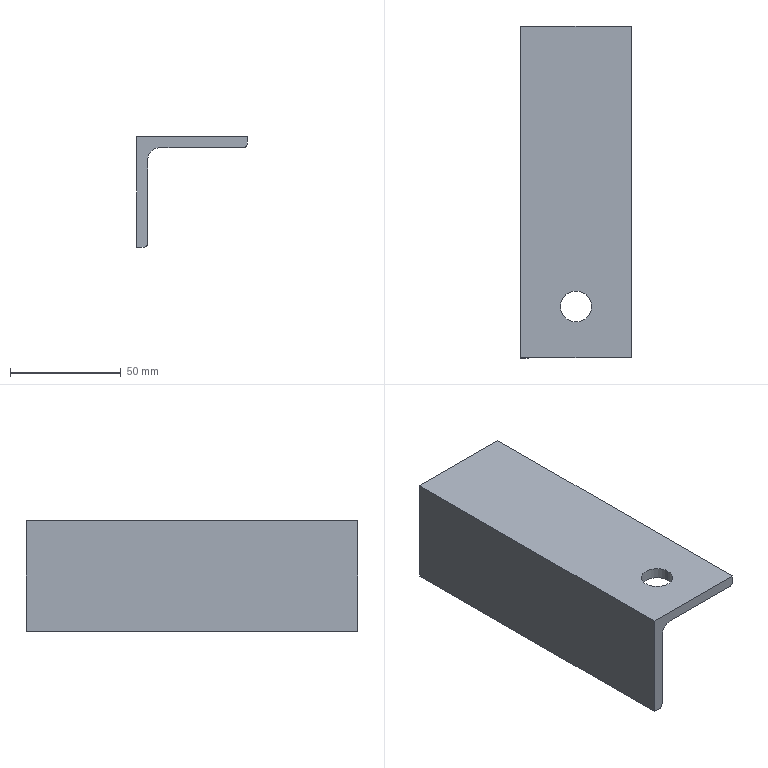Part | SolidWorks | features BaseBody 1 | 1 solid | 13 faces | box 50 x 150 x 50 mm | volume 71275 mm3 | plane 8 | cylinder 5 | commonest cylinder face diameters 3.333 x2 14 x2 11 x1
STEP:
#1=CARTESIAN_POINT('',(32.,-126.8,-5.));
#2=VERTEX_POINT('',#1);
#3=CARTESIAN_POINT('',(18.,-126.8,-5.));
#4=VERTEX_POINT('',#3);
#5=CARTESIAN_POINT('',(25.,-126.8,-5.));
#6=DIRECTION('',(0.,0.,-1.));
#7=DIRECTION('',(1.,0.,0.));
#8=AXIS2_PLACEMENT_3D('',#5,#6,#7);
#9=CIRCLE('',#8,7.);
#10=EDGE_CURVE('',#2,#4,#9,.T.);
#11=ORIENTED_EDGE('',*,*,#10,.T.);
#12=CARTESIAN_POINT('',(18.,-126.8,0.));
#13=VERTEX_POINT('',#12);
#14=CARTESIAN_POINT('',(18.,-126.8,-10.));
#15=DIRECTION('',(0.,0.,1.));
#16=VECTOR('',#15,1000.);
#17=LINE('',#14,#16);
#18=EDGE_CURVE('',#4,#13,#17,.T.);
#19=ORIENTED_EDGE('',*,*,#18,.T.);
#20=CARTESIAN_POINT('',(32.,-126.8,0.));
#21=VERTEX_POINT('',#20);
#22=CARTESIAN_POINT('',(25.,-126.8,0.));
#23=DIRECTION('',(0.,0.,1.));
#24=DIRECTION('',(1.,0.,0.));
#25=AXIS2_PLACEMENT_3D('',#22,#23,#24);
#26=CIRCLE('',#25,7.);
#27=EDGE_CURVE('',#13,#21,#26,.T.);
#28=ORIENTED_EDGE('',*,*,#27,.T.);
#29=CARTESIAN_POINT('',(32.,-126.8,-10.));
#30=DIRECTION('',(0.,0.,1.));
#31=VECTOR('',#30,1000.);
#32=LINE('',#29,#31);
#33=EDGE_CURVE('',#2,#21,#32,.T.);
#34=ORIENTED_EDGE('',*,*,#33,.F.);
#35=EDGE_LOOP('',(#11,#19,#28,#34));
#36=FACE_OUTER_BOUND('',#35,.T.);
#37=CARTESIAN_POINT('',(25.,-126.8,-10.));
#38=DIRECTION('',(0.,0.,1.));
#39=DIRECTION('',(1.,0.,0.));
#40=AXIS2_PLACEMENT_3D('',#37,#38,#39);
#41=CYLINDRICAL_SURFACE('',#40,7.);
#42=ADVANCED_FACE('',(#36),#41,.F.);
#43=CARTESIAN_POINT('',(0.,-150.,-50.));
#44=VERTEX_POINT('',#43);
#45=CARTESIAN_POINT('',(0.,0.,-50.));
#46=VERTEX_POINT('',#45);
#47=CARTESIAN_POINT('',(0.,-150.,-50.));
#48=DIRECTION('',(0.,1.,0.));
#49=VECTOR('',#48,1000.);
#50=LINE('',#47,#49);
#51=EDGE_CURVE('',#44,#46,#50,.T.);
#52=ORIENTED_EDGE('',*,*,#51,.F.);
#53=CARTESIAN_POINT('',(0.,-150.,0.));
#54=VERTEX_POINT('',#53);
#55=CARTESIAN_POINT('',(0.,-150.,0.));
#56=DIRECTION('',(0.,0.,-1.));
#57=VECTOR('',#56,1000.);
#58=LINE('',#55,#57);
#59=EDGE_CURVE('',#54,#44,#58,.T.);
#60=ORIENTED_EDGE('',*,*,#59,.F.);
#61=CARTESIAN_POINT('',(0.,0.,0.));
#62=VERTEX_POINT('',#61);
#63=CARTESIAN_POINT('',(0.,-150.,0.));
#64=DIRECTION('',(0.,-1.,0.));
#65=VECTOR('',#64,1000.);
#66=LINE('',#63,#65);
#67=EDGE_CURVE('',#62,#54,#66,.T.);
#68=ORIENTED_EDGE('',*,*,#67,.F.);
#69=CARTESIAN_POINT('',(0.,0.,0.));
#70=DIRECTION('',(0.,0.,1.));
#71=VECTOR('',#70,1000.);
#72=LINE('',#69,#71);
#73=EDGE_CURVE('',#46,#62,#72,.T.);
#74=ORIENTED_EDGE('',*,*,#73,.F.);
#75=EDGE_LOOP('',(#52,#60,#68,#74));
#76=FACE_OUTER_BOUND('',#75,.T.);
#77=CARTESIAN_POINT('',(0.,-150.,0.));
#78=DIRECTION('',(1.,0.,0.));
#79=DIRECTION('',(0.,1.,0.));
#80=AXIS2_PLACEMENT_3D('',#77,#78,#79);
#81=PLANE('',#80);
#82=ADVANCED_FACE('',(#76),#81,.F.);
#83=ORIENTED_EDGE('',*,*,#73,.T.);
#84=CARTESIAN_POINT('',(50.,0.,0.));
#85=VERTEX_POINT('',#84);
#86=CARTESIAN_POINT('',(48.333,0.,0.));
#87=DIRECTION('',(1.,0.,0.));
#88=VECTOR('',#87,1000.);
#89=LINE('',#86,#88);
#90=EDGE_CURVE('',#62,#85,#89,.T.);
#91=ORIENTED_EDGE('',*,*,#90,.T.);
#92=CARTESIAN_POINT('',(50.,0.,-3.333));
#93=VERTEX_POINT('',#92);
#94=CARTESIAN_POINT('',(50.,0.,-3.333));
#95=DIRECTION('',(0.,0.,-1.));
#96=VECTOR('',#95,1000.);
#97=LINE('',#94,#96);
#98=EDGE_CURVE('',#85,#93,#97,.T.);
#99=ORIENTED_EDGE('',*,*,#98,.T.);
#100=CARTESIAN_POINT('',(48.333,0.,-5.));
#101=VERTEX_POINT('',#100);
#102=CARTESIAN_POINT('',(48.333,0.,-3.333));
#103=DIRECTION('',(0.,1.,0.));
#104=DIRECTION('',(-1.,0.,0.));
#105=AXIS2_PLACEMENT_3D('',#102,#103,#104);
#106=CIRCLE('',#105,1.667);
#107=EDGE_CURVE('',#93,#101,#106,.T.);
#108=ORIENTED_EDGE('',*,*,#107,.T.);
#109=CARTESIAN_POINT('',(10.5,0.,-5.));
#110=VERTEX_POINT('',#109);
#111=CARTESIAN_POINT('',(48.333,0.,-5.));
#112=DIRECTION('',(-1.,0.,0.));
#113=VECTOR('',#112,1000.);
#114=LINE('',#111,#113);
#115=EDGE_CURVE('',#101,#110,#114,.T.);
#116=ORIENTED_EDGE('',*,*,#115,.T.);
#117=CARTESIAN_POINT('',(5.,0.,-10.5));
#118=VERTEX_POINT('',#117);
#119=CARTESIAN_POINT('',(10.5,0.,-10.5));
#120=DIRECTION('',(0.,-1.,0.));
#121=DIRECTION('',(-1.,0.,0.));
#122=AXIS2_PLACEMENT_3D('',#119,#120,#121);
#123=CIRCLE('',#122,5.5);
#124=EDGE_CURVE('',#110,#118,#123,.T.);
#125=ORIENTED_EDGE('',*,*,#124,.T.);
#126=CARTESIAN_POINT('',(5.,0.,-48.333));
#127=VERTEX_POINT('',#126);
#128=CARTESIAN_POINT('',(5.,0.,-3.333));
#129=DIRECTION('',(0.,0.,-1.));
#130=VECTOR('',#129,1000.);
#131=LINE('',#128,#130);
#132=EDGE_CURVE('',#118,#127,#131,.T.);
#133=ORIENTED_EDGE('',*,*,#132,.T.);
#134=CARTESIAN_POINT('',(3.333,0.,-50.));
#135=VERTEX_POINT('',#134);
#136=CARTESIAN_POINT('',(3.333,0.,-48.333));
#137=DIRECTION('',(0.,1.,0.));
#138=DIRECTION('',(-1.,0.,0.));
#139=AXIS2_PLACEMENT_3D('',#136,#137,#138);
#140=CIRCLE('',#139,1.667);
#141=EDGE_CURVE('',#127,#135,#140,.T.);
#142=ORIENTED_EDGE('',*,*,#141,.T.);
#143=CARTESIAN_POINT('',(48.333,0.,-50.));
#144=DIRECTION('',(-1.,0.,0.));
#145=VECTOR('',#144,1000.);
#146=LINE('',#143,#145);
#147=EDGE_CURVE('',#135,#46,#146,.T.);
#148=ORIENTED_EDGE('',*,*,#147,.T.);
#149=EDGE_LOOP('',(#83,#91,#99,#108,#116,#125,#133,#142,#148));
#150=FACE_OUTER_BOUND('',#149,.T.);
#151=CARTESIAN_POINT('',(48.333,0.,-3.333));
#152=DIRECTION('',(0.,1.,0.));
#153=DIRECTION('',(-1.,0.,0.));
#154=AXIS2_PLACEMENT_3D('',#151,#152,#153);
#155=PLANE('',#154);
#156=ADVANCED_FACE('',(#150),#155,.T.);
#157=CARTESIAN_POINT('',(3.333,-150.,-50.));
#158=VERTEX_POINT('',#157);
#159=CARTESIAN_POINT('',(3.333,-150.,-50.));
#160=DIRECTION('',(0.,1.,0.));
#161=VECTOR('',#160,1000.);
#162=LINE('',#159,#161);
#163=EDGE_CURVE('',#158,#135,#162,.T.);
#164=ORIENTED_EDGE('',*,*,#163,.F.);
#165=CARTESIAN_POINT('',(0.,-150.,-50.));
#166=DIRECTION('',(1.,0.,0.));
#167=VECTOR('',#166,1000.);
#168=LINE('',#165,#167);
#169=EDGE_CURVE('',#44,#158,#168,.T.);
#170=ORIENTED_EDGE('',*,*,#169,.F.);
#171=ORIENTED_EDGE('',*,*,#51,.T.);
#172=ORIENTED_EDGE('',*,*,#147,.F.);
#173=EDGE_LOOP('',(#164,#170,#171,#172));
#174=FACE_OUTER_BOUND('',#173,.T.);
#175=CARTESIAN_POINT('',(0.,-150.,-50.));
#176=DIRECTION('',(0.,0.,1.));
#177=DIRECTION('',(1.,0.,0.));
#178=AXIS2_PLACEMENT_3D('',#175,#176,#177);
#179=PLANE('',#178);
#180=ADVANCED_FACE('',(#174),#179,.F.);
#181=CARTESIAN_POINT('',(50.,-150.,0.));
#182=VERTEX_POINT('',#181);
#183=CARTESIAN_POINT('',(48.333,-150.,0.));
#184=DIRECTION('',(1.,0.,0.));
#185=VECTOR('',#184,1000.);
#186=LINE('',#183,#185);
#187=EDGE_CURVE('',#54,#182,#186,.T.);
#188=ORIENTED_EDGE('',*,*,#187,.F.);
#189=ORIENTED_EDGE('',*,*,#59,.T.);
#190=ORIENTED_EDGE('',*,*,#169,.T.);
#191=CARTESIAN_POINT('',(5.,-150.,-48.333));
#192=VERTEX_POINT('',#191);
#193=CARTESIAN_POINT('',(3.333,-150.,-48.333));
#194=DIRECTION('',(0.,1.,0.));
#195=DIRECTION('',(-1.,0.,0.));
#196=AXIS2_PLACEMENT_3D('',#193,#194,#195);
#197=CIRCLE('',#196,1.667);
#198=EDGE_CURVE('',#192,#158,#197,.T.);
#199=ORIENTED_EDGE('',*,*,#198,.F.);
#200=CARTESIAN_POINT('',(5.,-150.,-10.5));
#201=VERTEX_POINT('',#200);
#202=CARTESIAN_POINT('',(5.,-150.,-3.333));
#203=DIRECTION('',(0.,0.,-1.));
#204=VECTOR('',#203,1000.);
#205=LINE('',#202,#204);
#206=EDGE_CURVE('',#201,#192,#205,.T.);
#207=ORIENTED_EDGE('',*,*,#206,.F.);
#208=CARTESIAN_POINT('',(10.5,-150.,-5.));
#209=VERTEX_POINT('',#208);
#210=CARTESIAN_POINT('',(10.5,-150.,-10.5));
#211=DIRECTION('',(0.,-1.,0.));
#212=DIRECTION('',(-1.,0.,0.));
#213=AXIS2_PLACEMENT_3D('',#210,#211,#212);
#214=CIRCLE('',#213,5.5);
#215=EDGE_CURVE('',#209,#201,#214,.T.);
#216=ORIENTED_EDGE('',*,*,#215,.F.);
#217=CARTESIAN_POINT('',(48.333,-150.,-5.));
#218=VERTEX_POINT('',#217);
#219=CARTESIAN_POINT('',(48.333,-150.,-5.));
#220=DIRECTION('',(-1.,0.,0.));
#221=VECTOR('',#220,1000.);
#222=LINE('',#219,#221);
#223=EDGE_CURVE('',#218,#209,#222,.T.);
#224=ORIENTED_EDGE('',*,*,#223,.F.);
#225=CARTESIAN_POINT('',(50.,-150.,-3.333));
#226=VERTEX_POINT('',#225);
#227=CARTESIAN_POINT('',(48.333,-150.,-3.333));
#228=DIRECTION('',(0.,1.,0.));
#229=DIRECTION('',(-1.,0.,0.));
#230=AXIS2_PLACEMENT_3D('',#227,#228,#229);
#231=CIRCLE('',#230,1.667);
#232=EDGE_CURVE('',#226,#218,#231,.T.);
#233=ORIENTED_EDGE('',*,*,#232,.F.);
#234=CARTESIAN_POINT('',(50.,-150.,-3.333));
#235=DIRECTION('',(0.,0.,-1.));
#236=VECTOR('',#235,1000.);
#237=LINE('',#234,#236);
#238=EDGE_CURVE('',#182,#226,#237,.T.);
#239=ORIENTED_EDGE('',*,*,#238,.F.);
#240=EDGE_LOOP('',(#188,#189,#190,#199,#207,#216,#224,#233,#239));
#241=FACE_OUTER_BOUND('',#240,.T.);
#242=CARTESIAN_POINT('',(48.333,-150.,-3.333));
#243=DIRECTION('',(0.,1.,0.));
#244=DIRECTION('',(-1.,0.,0.));
#245=AXIS2_PLACEMENT_3D('',#242,#243,#244);
#246=PLANE('',#245);
#247=ADVANCED_FACE('',(#241),#246,.F.);
#248=ORIENTED_EDGE('',*,*,#67,.T.);
#249=ORIENTED_EDGE('',*,*,#187,.T.);
#250=CARTESIAN_POINT('',(50.,-150.,0.));
#251=DIRECTION('',(0.,-1.,0.));
#252=VECTOR('',#251,1000.);
#253=LINE('',#250,#252);
#254=EDGE_CURVE('',#85,#182,#253,.T.);
#255=ORIENTED_EDGE('',*,*,#254,.F.);
#256=ORIENTED_EDGE('',*,*,#90,.F.);
#257=EDGE_LOOP('',(#248,#249,#255,#256));
#258=FACE_OUTER_BOUND('',#257,.T.);
#259=CARTESIAN_POINT('',(25.,-126.8,0.));
#260=DIRECTION('',(0.,0.,1.));
#261=DIRECTION('',(1.,0.,0.));
#262=AXIS2_PLACEMENT_3D('',#259,#260,#261);
#263=CIRCLE('',#262,7.);
#264=EDGE_CURVE('',#21,#13,#263,.T.);
#265=ORIENTED_EDGE('',*,*,#264,.F.);
#266=ORIENTED_EDGE('',*,*,#27,.F.);
#267=EDGE_LOOP('',(#265,#266));
#268=FACE_BOUND('',#267,.T.);
#269=CARTESIAN_POINT('',(50.,-150.,0.));
#270=DIRECTION('',(0.,0.,-1.));
#271=DIRECTION('',(-1.,0.,0.));
#272=AXIS2_PLACEMENT_3D('',#269,#270,#271);
#273=PLANE('',#272);
#274=ADVANCED_FACE('',(#258,#268),#273,.F.);
#275=ORIENTED_EDGE('',*,*,#198,.T.);
#276=ORIENTED_EDGE('',*,*,#163,.T.);
#277=ORIENTED_EDGE('',*,*,#141,.F.);
#278=CARTESIAN_POINT('',(5.,-150.,-48.333));
#279=DIRECTION('',(0.,-1.,0.));
#280=VECTOR('',#279,1000.);
#281=LINE('',#278,#280);
#282=EDGE_CURVE('',#127,#192,#281,.T.);
#283=ORIENTED_EDGE('',*,*,#282,.T.);
#284=EDGE_LOOP('',(#275,#276,#277,#283));
#285=FACE_OUTER_BOUND('',#284,.T.);
#286=CARTESIAN_POINT('',(3.333,-150.,-48.333));
#287=DIRECTION('',(0.,1.,0.));
#288=DIRECTION('',(-1.,0.,0.));
#289=AXIS2_PLACEMENT_3D('',#286,#287,#288);
#290=CYLINDRICAL_SURFACE('',#289,1.667);
#291=ADVANCED_FACE('',(#285),#290,.T.);
#292=CARTESIAN_POINT('',(5.,-150.,-10.5));
#293=DIRECTION('',(0.,1.,0.));
#294=VECTOR('',#293,1000.);
#295=LINE('',#292,#294);
#296=EDGE_CURVE('',#201,#118,#295,.T.);
#297=ORIENTED_EDGE('',*,*,#296,.F.);
#298=ORIENTED_EDGE('',*,*,#206,.T.);
#299=ORIENTED_EDGE('',*,*,#282,.F.);
#300=ORIENTED_EDGE('',*,*,#132,.F.);
#301=EDGE_LOOP('',(#297,#298,#299,#300));
#302=FACE_OUTER_BOUND('',#301,.T.);
#303=CARTESIAN_POINT('',(5.,-150.,-10.5));
#304=DIRECTION('',(-1.,0.,0.));
#305=DIRECTION('',(0.,-1.,0.));
#306=AXIS2_PLACEMENT_3D('',#303,#304,#305);
#307=PLANE('',#306);
#308=ADVANCED_FACE('',(#302),#307,.F.);
#309=CARTESIAN_POINT('',(10.5,-150.,-5.));
#310=DIRECTION('',(0.,1.,0.));
#311=VECTOR('',#310,1000.);
#312=LINE('',#309,#311);
#313=EDGE_CURVE('',#209,#110,#312,.T.);
#314=ORIENTED_EDGE('',*,*,#313,.F.);
#315=ORIENTED_EDGE('',*,*,#215,.T.);
#316=ORIENTED_EDGE('',*,*,#296,.T.);
#317=ORIENTED_EDGE('',*,*,#124,.F.);
#318=EDGE_LOOP('',(#314,#315,#316,#317));
#319=FACE_OUTER_BOUND('',#318,.T.);
#320=CARTESIAN_POINT('',(10.5,-150.,-10.5));
#321=DIRECTION('',(0.,1.,0.));
#322=DIRECTION('',(-1.,0.,0.));
#323=AXIS2_PLACEMENT_3D('',#320,#321,#322);
#324=CYLINDRICAL_SURFACE('',#323,5.5);
#325=ADVANCED_FACE('',(#319),#324,.F.);
#326=CARTESIAN_POINT('',(48.333,-150.,-5.));
#327=DIRECTION('',(0.,1.,0.));
#328=VECTOR('',#327,1000.);
#329=LINE('',#326,#328);
#330=EDGE_CURVE('',#218,#101,#329,.T.);
#331=ORIENTED_EDGE('',*,*,#330,.F.);
#332=ORIENTED_EDGE('',*,*,#223,.T.);
#333=ORIENTED_EDGE('',*,*,#313,.T.);
#334=ORIENTED_EDGE('',*,*,#115,.F.);
#335=EDGE_LOOP('',(#331,#332,#333,#334));
#336=FACE_OUTER_BOUND('',#335,.T.);
#337=ORIENTED_EDGE('',*,*,#10,.F.);
#338=CARTESIAN_POINT('',(25.,-126.8,-5.));
#339=DIRECTION('',(0.,0.,-1.));
#340=DIRECTION('',(1.,0.,0.));
#341=AXIS2_PLACEMENT_3D('',#338,#339,#340);
#342=CIRCLE('',#341,7.);
#343=EDGE_CURVE('',#4,#2,#342,.T.);
#344=ORIENTED_EDGE('',*,*,#343,.F.);
#345=EDGE_LOOP('',(#337,#344));
#346=FACE_BOUND('',#345,.T.);
#347=CARTESIAN_POINT('',(48.333,-150.,-5.));
#348=DIRECTION('',(0.,0.,1.));
#349=DIRECTION('',(1.,0.,0.));
#350=AXIS2_PLACEMENT_3D('',#347,#348,#349);
#351=PLANE('',#350);
#352=ADVANCED_FACE('',(#336,#346),#351,.F.);
#353=ORIENTED_EDGE('',*,*,#232,.T.);
#354=ORIENTED_EDGE('',*,*,#330,.T.);
#355=ORIENTED_EDGE('',*,*,#107,.F.);
#356=CARTESIAN_POINT('',(50.,-150.,-3.333));
#357=DIRECTION('',(0.,-1.,0.));
#358=VECTOR('',#357,1000.);
#359=LINE('',#356,#358);
#360=EDGE_CURVE('',#93,#226,#359,.T.);
#361=ORIENTED_EDGE('',*,*,#360,.T.);
#362=EDGE_LOOP('',(#353,#354,#355,#361));
#363=FACE_OUTER_BOUND('',#362,.T.);
#364=CARTESIAN_POINT('',(48.333,-150.,-3.333));
#365=DIRECTION('',(0.,1.,0.));
#366=DIRECTION('',(-1.,0.,0.));
#367=AXIS2_PLACEMENT_3D('',#364,#365,#366);
#368=CYLINDRICAL_SURFACE('',#367,1.667);
#369=ADVANCED_FACE('',(#363),#368,.T.);
#370=ORIENTED_EDGE('',*,*,#254,.T.);
#371=ORIENTED_EDGE('',*,*,#238,.T.);
#372=ORIENTED_EDGE('',*,*,#360,.F.);
#373=ORIENTED_EDGE('',*,*,#98,.F.);
#374=EDGE_LOOP('',(#370,#371,#372,#373));
#375=FACE_OUTER_BOUND('',#374,.T.);
#376=CARTESIAN_POINT('',(50.,-150.,0.));
#377=DIRECTION('',(-1.,0.,0.));
#378=DIRECTION('',(0.,-1.,0.));
#379=AXIS2_PLACEMENT_3D('',#376,#377,#378);
#380=PLANE('',#379);
#381=ADVANCED_FACE('',(#375),#380,.F.);
#382=ORIENTED_EDGE('',*,*,#18,.F.);
#383=ORIENTED_EDGE('',*,*,#343,.T.);
#384=ORIENTED_EDGE('',*,*,#33,.T.);
#385=ORIENTED_EDGE('',*,*,#264,.T.);
#386=EDGE_LOOP('',(#382,#383,#384,#385));
#387=FACE_OUTER_BOUND('',#386,.T.);
#388=CARTESIAN_POINT('',(25.,-126.8,-10.));
#389=DIRECTION('',(0.,0.,1.));
#390=DIRECTION('',(1.,0.,0.));
#391=AXIS2_PLACEMENT_3D('',#388,#389,#390);
#392=CYLINDRICAL_SURFACE('',#391,7.);
#393=ADVANCED_FACE('',(#387),#392,.F.);
#394=CLOSED_SHELL('',(#42,#82,#156,#180,#247,#274,#291,#308,#325,#352,#369,#381,#393));
#395=MANIFOLD_SOLID_BREP('',#394);
#396=CARTESIAN_POINT('',(0.,0.,0.));
#397=DIRECTION('',(0.,0.,1.));
#398=DIRECTION('',(1.,0.,0.));
#399=AXIS2_PLACEMENT_3D('',#396,#397,#398);
#400=(LENGTH_UNIT()NAMED_UNIT(*)SI_UNIT(.MILLI.,.METRE.));
#401=UNCERTAINTY_MEASURE_WITH_UNIT(LENGTH_MEASURE(0.00001),#400,'','');
#402=(NAMED_UNIT(*)PLANE_ANGLE_UNIT()SI_UNIT($,.RADIAN.));
#403=(NAMED_UNIT(*)SI_UNIT($,.STERADIAN.)SOLID_ANGLE_UNIT());
#404=(GEOMETRIC_REPRESENTATION_CONTEXT(3)GLOBAL_UNCERTAINTY_ASSIGNED_CONTEXT((#401))GLOBAL_UNIT_ASSIGNED_CONTEXT((#400,#402,#403))REPRESENTATION_CONTEXT('',''));
#405=ADVANCED_BREP_SHAPE_REPRESENTATION('',(#395,#399),#404);